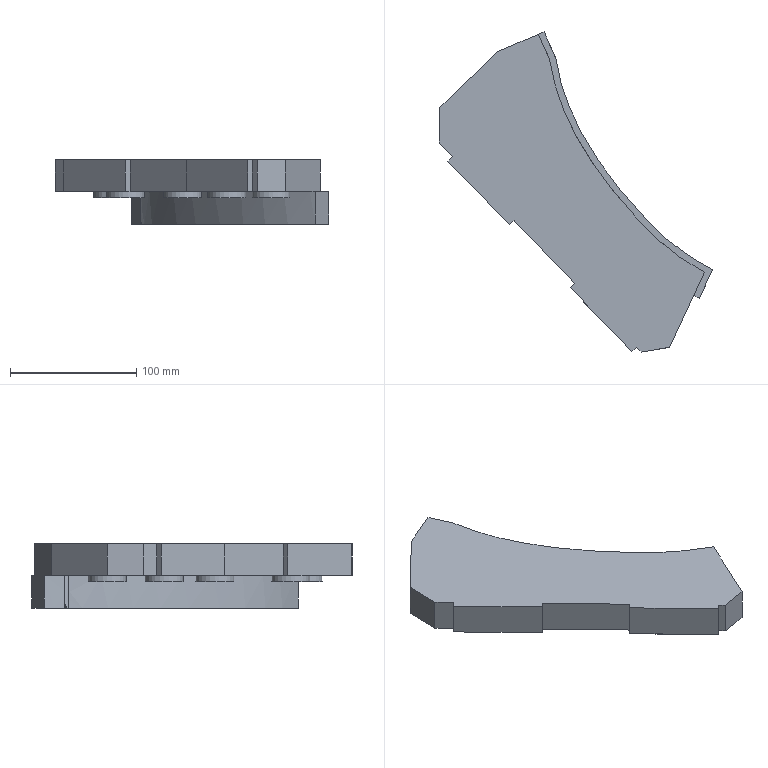Part | NX | features solid 2 | 1 solid | 32 faces | box 216.104 x 253.124 x 51 mm | volume 711831 mm3 | plane 24 | cylinder 5 | spline 3 | commonest cylinder face diameters 30 x5
STEP:
#1=CARTESIAN_POINT('',(-720.611,-200.558,20.));
#2=VERTEX_POINT('',#1);
#3=CARTESIAN_POINT('',(-705.611,-200.558,20.));
#4=DIRECTION('',(0.,0.,-1.));
#5=DIRECTION('',(-1.,0.,0.));
#6=AXIS2_PLACEMENT_3D('',#3,#4,#5);
#7=CIRCLE('',#6,15.);
#8=EDGE_CURVE('',#2,#2,#7,.T.);
#9=ORIENTED_EDGE('',*,*,#8,.F.);
#10=EDGE_LOOP('',(#9));
#11=FACE_BOUND('',#10,.T.);
#12=CARTESIAN_POINT('',(-640.003,-204.168,20.));
#13=VERTEX_POINT('',#12);
#14=CARTESIAN_POINT('',(-659.197,-245.33,20.));
#15=VERTEX_POINT('',#14);
#16=CARTESIAN_POINT('',(-631.647,-186.248,20.));
#17=DIRECTION('',(0.4226,0.9063,0.));
#18=VECTOR('',#17,1000.);
#19=LINE('',#16,#18);
#20=EDGE_CURVE('',#13,#15,#19,.F.);
#21=ORIENTED_EDGE('',*,*,#20,.T.);
#22=CARTESIAN_POINT('',(-681.543,-249.069,20.));
#23=VERTEX_POINT('',#22);
#24=CARTESIAN_POINT('',(-659.197,-245.33,20.));
#25=DIRECTION('',(0.9863,0.165,0.));
#26=VECTOR('',#25,1000.);
#27=LINE('',#24,#26);
#28=EDGE_CURVE('',#15,#23,#27,.F.);
#29=ORIENTED_EDGE('',*,*,#28,.T.);
#30=CARTESIAN_POINT('',(-685.314,-245.163,20.));
#31=VERTEX_POINT('',#30);
#32=CARTESIAN_POINT('',(-646.435,-285.424,20.));
#33=DIRECTION('',(0.6947,-0.7193,0.));
#34=VECTOR('',#33,1000.);
#35=LINE('',#32,#34);
#36=EDGE_CURVE('',#23,#31,#35,.F.);
#37=ORIENTED_EDGE('',*,*,#36,.T.);
#38=CARTESIAN_POINT('',(-688.911,-248.636,20.));
#39=VERTEX_POINT('',#38);
#40=CARTESIAN_POINT('',(-604.539,-167.159,20.));
#41=DIRECTION('',(0.7193,0.6947,0.));
#42=VECTOR('',#41,1000.);
#43=LINE('',#40,#42);
#44=EDGE_CURVE('',#31,#39,#43,.F.);
#45=ORIENTED_EDGE('',*,*,#44,.T.);
#46=CARTESIAN_POINT('',(-737.537,-198.283,20.));
#47=VERTEX_POINT('',#46);
#48=CARTESIAN_POINT('',(-661.125,-277.41,20.));
#49=DIRECTION('',(0.6947,-0.7193,0.));
#50=VECTOR('',#49,1000.);
#51=LINE('',#48,#50);
#52=EDGE_CURVE('',#47,#39,#51,.T.);
#53=ORIENTED_EDGE('',*,*,#52,.F.);
#54=CARTESIAN_POINT('',(-733.94,-194.809,20.));
#55=VERTEX_POINT('',#54);
#56=CARTESIAN_POINT('',(-653.165,-116.805,20.));
#57=DIRECTION('',(0.7193,0.6947,0.));
#58=VECTOR('',#57,1000.);
#59=LINE('',#56,#58);
#60=EDGE_CURVE('',#55,#47,#59,.F.);
#61=ORIENTED_EDGE('',*,*,#60,.F.);
#62=CARTESIAN_POINT('',(-782.058,-144.982,20.));
#63=VERTEX_POINT('',#62);
#64=CARTESIAN_POINT('',(-646.435,-285.424,20.));
#65=DIRECTION('',(0.6947,-0.7193,0.));
#66=VECTOR('',#65,1000.);
#67=LINE('',#64,#66);
#68=EDGE_CURVE('',#55,#63,#67,.F.);
#69=ORIENTED_EDGE('',*,*,#68,.T.);
#70=CARTESIAN_POINT('',(-785.655,-148.455,20.));
#71=VERTEX_POINT('',#70);
#72=CARTESIAN_POINT('',(-701.283,-66.978,20.));
#73=DIRECTION('',(0.7193,0.6947,0.));
#74=VECTOR('',#73,1000.);
#75=LINE('',#72,#74);
#76=EDGE_CURVE('',#63,#71,#75,.F.);
#77=ORIENTED_EDGE('',*,*,#76,.T.);
#78=CARTESIAN_POINT('',(-834.281,-98.101,20.));
#79=VERTEX_POINT('',#78);
#80=CARTESIAN_POINT('',(-837.754,-94.505,20.));
#81=DIRECTION('',(0.6947,-0.7193,0.));
#82=VECTOR('',#81,1000.);
#83=LINE('',#80,#82);
#84=EDGE_CURVE('',#79,#71,#83,.T.);
#85=ORIENTED_EDGE('',*,*,#84,.F.);
#86=CARTESIAN_POINT('',(-830.684,-94.628,20.));
#87=VERTEX_POINT('',#86);
#88=CARTESIAN_POINT('',(-749.909,-16.624,20.));
#89=DIRECTION('',(0.7193,0.6947,0.));
#90=VECTOR('',#89,1000.);
#91=LINE('',#88,#90);
#92=EDGE_CURVE('',#87,#79,#91,.F.);
#93=ORIENTED_EDGE('',*,*,#92,.F.);
#94=CARTESIAN_POINT('',(-841.104,-83.838,20.));
#95=VERTEX_POINT('',#94);
#96=CARTESIAN_POINT('',(-646.435,-285.424,20.));
#97=DIRECTION('',(0.6947,-0.7193,0.));
#98=VECTOR('',#97,1000.);
#99=LINE('',#96,#98);
#100=EDGE_CURVE('',#87,#95,#99,.F.);
#101=ORIENTED_EDGE('',*,*,#100,.T.);
#102=CARTESIAN_POINT('',(-840.611,-55.558,20.));
#103=VERTEX_POINT('',#102);
#104=CARTESIAN_POINT('',(-841.104,-83.838,20.));
#105=DIRECTION('',(0.01745,0.9998,0.));
#106=VECTOR('',#105,1000.);
#107=LINE('',#104,#106);
#108=EDGE_CURVE('',#95,#103,#107,.T.);
#109=ORIENTED_EDGE('',*,*,#108,.T.);
#110=CARTESIAN_POINT('',(-795.068,-11.578,20.));
#111=VERTEX_POINT('',#110);
#112=CARTESIAN_POINT('',(-774.222,8.553,20.));
#113=DIRECTION('',(-0.7193,-0.6947,0.));
#114=VECTOR('',#113,1000.);
#115=LINE('',#112,#114);
#116=EDGE_CURVE('',#103,#111,#115,.F.);
#117=ORIENTED_EDGE('',*,*,#116,.T.);
#118=CARTESIAN_POINT('',(-781.258,-5.716,20.));
#119=VERTEX_POINT('',#118);
#120=CARTESIAN_POINT('',(-1958.229,-505.311,20.));
#121=DIRECTION('',(-0.9205,-0.3907,0.));
#122=VECTOR('',#121,1000.);
#123=LINE('',#120,#122);
#124=EDGE_CURVE('',#111,#119,#123,.F.);
#125=ORIENTED_EDGE('',*,*,#124,.T.);
#126=CARTESIAN_POINT('',(-640.003,-204.168,20.));
#127=CARTESIAN_POINT('',(-649.16,-199.229,20.));
#128=CARTESIAN_POINT('',(-658.155,-193.671,20.));
#129=CARTESIAN_POINT('',(-674.999,-181.298,20.));
#130=CARTESIAN_POINT('',(-682.803,-174.446,20.));
#131=CARTESIAN_POINT('',(-697.433,-159.689,20.));
#132=CARTESIAN_POINT('',(-704.434,-151.972,20.));
#133=CARTESIAN_POINT('',(-718.006,-136.075,20.));
#134=CARTESIAN_POINT('',(-724.478,-127.917,20.));
#135=CARTESIAN_POINT('',(-736.62,-111.085,20.));
#136=CARTESIAN_POINT('',(-742.292,-102.411,20.));
#137=CARTESIAN_POINT('',(-752.624,-84.404,20.));
#138=CARTESIAN_POINT('',(-757.308,-75.035,20.));
#139=CARTESIAN_POINT('',(-765.276,-55.633,20.));
#140=CARTESIAN_POINT('',(-768.539,-45.674,20.));
#141=CARTESIAN_POINT('',(-771.484,-32.818,20.));
#142=CARTESIAN_POINT('',(-772.016,-30.226,20.));
#143=CARTESIAN_POINT('',(-772.603,-26.959,20.));
#144=CARTESIAN_POINT('',(-772.774,-25.976,20.));
#145=CARTESIAN_POINT('',(-772.936,-24.991,20.));
#146=CARTESIAN_POINT('',(-773.042,-24.334,20.));
#147=CARTESIAN_POINT('',(-773.052,-23.989,20.));
#148=CARTESIAN_POINT('',(-773.753,-22.502,20.));
#149=CARTESIAN_POINT('',(-774.301,-21.307,20.));
#150=CARTESIAN_POINT('',(-777.083,-15.349,20.));
#151=CARTESIAN_POINT('',(-779.311,-10.583,20.));
#152=CARTESIAN_POINT('',(-781.258,-5.716,20.));
#153=B_SPLINE_CURVE_WITH_KNOTS('',3,(#126,#127,#128,#129,#130,#131,#132,#133,#134,#135,#136,#137,#138,#139,#140,#141,#142,#143,#144,#145,#146,#147,#148,#149,#150,#151,#152),.UNSPECIFIED.,.F.,.F.,(4,2,2,2,2,2,2,2,2,1,2,2,2,4),(0.,0.125,0.25,0.375,0.5,0.625,0.75,0.875,0.9062,0.9141,0.918,0.9219,0.9375,1.),.UNSPECIFIED.);
#154=EDGE_CURVE('',#13,#119,#153,.T.);
#155=ORIENTED_EDGE('',*,*,#154,.F.);
#156=EDGE_LOOP('',(#21,#29,#37,#45,#53,#61,#69,#77,#85,#93,#101,#109,#117,#125,#155));
#157=FACE_BOUND('',#156,.T.);
#158=CARTESIAN_POINT('',(-770.611,-100.558,20.));
#159=VERTEX_POINT('',#158);
#160=CARTESIAN_POINT('',(-785.611,-100.558,20.));
#161=DIRECTION('',(0.,0.,1.));
#162=DIRECTION('',(1.,0.,0.));
#163=AXIS2_PLACEMENT_3D('',#160,#161,#162);
#164=CIRCLE('',#163,15.);
#165=EDGE_CURVE('',#159,#159,#164,.T.);
#166=ORIENTED_EDGE('',*,*,#165,.T.);
#167=EDGE_LOOP('',(#166));
#168=FACE_BOUND('',#167,.T.);
#169=CARTESIAN_POINT('',(-780.611,-55.558,20.));
#170=VERTEX_POINT('',#169);
#171=CARTESIAN_POINT('',(-795.611,-55.558,20.));
#172=DIRECTION('',(0.,0.,1.));
#173=DIRECTION('',(1.,0.,0.));
#174=AXIS2_PLACEMENT_3D('',#171,#172,#173);
#175=CIRCLE('',#174,15.);
#176=EDGE_CURVE('',#170,#170,#175,.T.);
#177=ORIENTED_EDGE('',*,*,#176,.T.);
#178=EDGE_LOOP('',(#177));
#179=FACE_BOUND('',#178,.T.);
#180=CARTESIAN_POINT('',(-755.611,-140.558,20.));
#181=VERTEX_POINT('',#180);
#182=CARTESIAN_POINT('',(-740.611,-140.558,20.));
#183=DIRECTION('',(0.,0.,-1.));
#184=DIRECTION('',(-1.,0.,0.));
#185=AXIS2_PLACEMENT_3D('',#182,#183,#184);
#186=CIRCLE('',#185,15.);
#187=EDGE_CURVE('',#181,#181,#186,.T.);
#188=ORIENTED_EDGE('',*,*,#187,.F.);
#189=EDGE_LOOP('',(#188));
#190=FACE_BOUND('',#189,.T.);
#191=CARTESIAN_POINT('',(-685.611,-210.558,20.));
#192=VERTEX_POINT('',#191);
#193=CARTESIAN_POINT('',(-670.611,-210.558,20.));
#194=DIRECTION('',(0.,0.,-1.));
#195=DIRECTION('',(-1.,0.,0.));
#196=AXIS2_PLACEMENT_3D('',#193,#194,#195);
#197=CIRCLE('',#196,15.);
#198=EDGE_CURVE('',#192,#192,#197,.T.);
#199=ORIENTED_EDGE('',*,*,#198,.F.);
#200=EDGE_LOOP('',(#199));
#201=FACE_BOUND('',#200,.T.);
#202=CARTESIAN_POINT('',(-565.659,-207.42,20.));
#203=DIRECTION('',(0.,0.,-1.));
#204=DIRECTION('',(-1.,0.,0.));
#205=AXIS2_PLACEMENT_3D('',#202,#203,#204);
#206=PLANE('',#205);
#207=ADVANCED_FACE('',(#11,#157,#168,#179,#190,#201),#206,.T.);
#208=CARTESIAN_POINT('',(-631.535,-186.008,20.));
#209=VERTEX_POINT('',#208);
#210=CARTESIAN_POINT('',(-631.535,-186.008,45.));
#211=VERTEX_POINT('',#210);
#212=CARTESIAN_POINT('',(-631.535,-186.008,32.5));
#213=DIRECTION('',(0.,0.,-1.));
#214=VECTOR('',#213,1000.);
#215=LINE('',#212,#214);
#216=EDGE_CURVE('',#209,#211,#215,.F.);
#217=ORIENTED_EDGE('',*,*,#216,.F.);
#218=CARTESIAN_POINT('',(-762.843,2.1,20.));
#219=VERTEX_POINT('',#218);
#220=CARTESIAN_POINT('',(-631.535,-186.008,20.));
#221=CARTESIAN_POINT('',(-635.789,-183.687,20.));
#222=CARTESIAN_POINT('',(-644.159,-178.788,20.));
#223=CARTESIAN_POINT('',(-656.221,-170.521,20.));
#224=CARTESIAN_POINT('',(-667.69,-161.153,20.));
#225=CARTESIAN_POINT('',(-678.201,-150.812,20.));
#226=CARTESIAN_POINT('',(-688.244,-139.998,20.));
#227=CARTESIAN_POINT('',(-701.112,-125.267,20.));
#228=CARTESIAN_POINT('',(-713.112,-109.922,20.));
#229=CARTESIAN_POINT('',(-723.992,-93.811,20.));
#230=CARTESIAN_POINT('',(-731.511,-81.281,20.));
#231=CARTESIAN_POINT('',(-738.298,-68.261,20.));
#232=CARTESIAN_POINT('',(-743.263,-56.884,20.));
#233=CARTESIAN_POINT('',(-746.689,-47.546,20.));
#234=CARTESIAN_POINT('',(-748.961,-40.442,20.));
#235=CARTESIAN_POINT('',(-750.591,-34.427,20.));
#236=CARTESIAN_POINT('',(-751.722,-29.553,20.));
#237=CARTESIAN_POINT('',(-752.488,-25.868,20.));
#238=CARTESIAN_POINT('',(-753.027,-22.762,20.));
#239=CARTESIAN_POINT('',(-753.46,-20.278,20.));
#240=CARTESIAN_POINT('',(-753.634,-18.362,20.));
#241=CARTESIAN_POINT('',(-754.376,-16.647,20.));
#242=CARTESIAN_POINT('',(-755.479,-14.402,20.));
#243=CARTESIAN_POINT('',(-756.769,-11.564,20.));
#244=CARTESIAN_POINT('',(-758.364,-8.175,20.));
#245=CARTESIAN_POINT('',(-760.444,-3.64,20.));
#246=CARTESIAN_POINT('',(-761.927,-0.2114,20.));
#247=CARTESIAN_POINT('',(-762.843,2.1,20.));
#248=B_SPLINE_CURVE_WITH_KNOTS('',3,(#220,#221,#222,#223,#224,#225,#226,#227,#228,#229,#230,#231,#232,#233,#234,#235,#236,#237,#238,#239,#240,#241,#242,#243,#244,#245,#246,#247),.UNSPECIFIED.,.F.,.F.,(4,1,1,1,1,1,1,1,1,1,1,1,1,1,1,1,1,1,1,1,1,1,1,1,1,4),(0.7404,0.7551,0.7697,0.7844,0.7991,0.8137,0.8284,0.8577,0.8724,0.887,0.9017,0.9163,0.9237,0.931,0.9383,0.942,0.9456,0.9493,0.9511,0.953,0.9548,0.9566,0.9603,0.964,0.9676,0.975),.UNSPECIFIED.);
#249=EDGE_CURVE('',#209,#219,#248,.T.);
#250=ORIENTED_EDGE('',*,*,#249,.T.);
#251=CARTESIAN_POINT('',(-762.843,2.1,45.));
#252=VERTEX_POINT('',#251);
#253=CARTESIAN_POINT('',(-762.843,2.1,42.5));
#254=DIRECTION('',(0.,0.,-1.));
#255=VECTOR('',#254,1000.);
#256=LINE('',#253,#255);
#257=EDGE_CURVE('',#219,#252,#256,.F.);
#258=ORIENTED_EDGE('',*,*,#257,.T.);
#259=CARTESIAN_POINT('',(-631.535,-186.008,45.));
#260=CARTESIAN_POINT('',(-635.79,-183.686,45.));
#261=CARTESIAN_POINT('',(-644.175,-178.778,45.));
#262=CARTESIAN_POINT('',(-656.267,-170.491,45.));
#263=CARTESIAN_POINT('',(-667.861,-161.004,45.));
#264=CARTESIAN_POINT('',(-678.395,-150.608,45.));
#265=CARTESIAN_POINT('',(-688.433,-139.79,45.));
#266=CARTESIAN_POINT('',(-701.359,-124.97,45.));
#267=CARTESIAN_POINT('',(-713.457,-109.469,45.));
#268=CARTESIAN_POINT('',(-724.514,-93.,45.));
#269=CARTESIAN_POINT('',(-732.09,-80.249,45.));
#270=CARTESIAN_POINT('',(-738.81,-67.179,45.));
#271=CARTESIAN_POINT('',(-743.63,-55.962,45.));
#272=CARTESIAN_POINT('',(-746.951,-46.773,45.));
#273=CARTESIAN_POINT('',(-749.158,-39.765,45.));
#274=CARTESIAN_POINT('',(-750.742,-33.822,45.));
#275=CARTESIAN_POINT('',(-751.843,-28.999,45.));
#276=CARTESIAN_POINT('',(-752.584,-25.348,45.));
#277=CARTESIAN_POINT('',(-753.119,-22.271,45.));
#278=CARTESIAN_POINT('',(-753.516,-19.798,45.));
#279=CARTESIAN_POINT('',(-753.755,-17.918,45.));
#280=CARTESIAN_POINT('',(-754.577,-16.276,45.));
#281=CARTESIAN_POINT('',(-755.62,-14.066,45.));
#282=CARTESIAN_POINT('',(-756.901,-11.293,45.));
#283=CARTESIAN_POINT('',(-758.457,-7.973,45.));
#284=CARTESIAN_POINT('',(-760.493,-3.531,45.));
#285=CARTESIAN_POINT('',(-761.944,-0.169,45.));
#286=CARTESIAN_POINT('',(-762.843,2.1,45.));
#287=B_SPLINE_CURVE_WITH_KNOTS('',3,(#259,#260,#261,#262,#263,#264,#265,#266,#267,#268,#269,#270,#271,#272,#273,#274,#275,#276,#277,#278,#279,#280,#281,#282,#283,#284,#285,#286),.UNSPECIFIED.,.F.,.F.,(4,1,1,1,1,1,1,1,1,1,1,1,1,1,1,1,1,1,1,1,1,1,1,1,1,4),(0.06935,0.08388,0.09841,0.1129,0.1275,0.142,0.1565,0.1856,0.2001,0.2147,0.2292,0.2437,0.251,0.2583,0.2655,0.2692,0.2728,0.2764,0.2782,0.2801,0.2819,0.2837,0.2873,0.291,0.2946,0.3019),.UNSPECIFIED.);
#288=EDGE_CURVE('',#211,#252,#287,.T.);
#289=ORIENTED_EDGE('',*,*,#288,.F.);
#290=EDGE_LOOP('',(#217,#250,#258,#289));
#291=FACE_BOUND('',#290,.T.);
#292=CARTESIAN_POINT('',(-631.535,-186.008,45.));
#293=CARTESIAN_POINT('',(-631.535,-186.008,20.));
#294=CARTESIAN_POINT('',(-635.877,-183.639,45.));
#295=CARTESIAN_POINT('',(-635.877,-183.639,20.));
#296=CARTESIAN_POINT('',(-644.43,-178.626,45.));
#297=CARTESIAN_POINT('',(-644.43,-178.626,20.));
#298=CARTESIAN_POINT('',(-656.738,-170.143,45.));
#299=CARTESIAN_POINT('',(-656.738,-170.143,20.));
#300=CARTESIAN_POINT('',(-668.325,-160.586,45.));
#301=CARTESIAN_POINT('',(-668.325,-160.586,20.));
#302=CARTESIAN_POINT('',(-678.899,-150.079,45.));
#303=CARTESIAN_POINT('',(-678.899,-150.079,20.));
#304=CARTESIAN_POINT('',(-688.858,-139.317,45.));
#305=CARTESIAN_POINT('',(-688.858,-139.317,20.));
#306=CARTESIAN_POINT('',(-701.731,-124.516,45.));
#307=CARTESIAN_POINT('',(-701.731,-124.516,20.));
#308=CARTESIAN_POINT('',(-713.804,-108.992,45.));
#309=CARTESIAN_POINT('',(-713.804,-108.992,20.));
#310=CARTESIAN_POINT('',(-724.771,-92.591,45.));
#311=CARTESIAN_POINT('',(-724.771,-92.591,20.));
#312=CARTESIAN_POINT('',(-732.323,-79.832,45.));
#313=CARTESIAN_POINT('',(-732.323,-79.832,20.));
#314=CARTESIAN_POINT('',(-739.096,-66.587,45.));
#315=CARTESIAN_POINT('',(-739.096,-66.587,20.));
#316=CARTESIAN_POINT('',(-743.961,-55.141,45.));
#317=CARTESIAN_POINT('',(-743.961,-55.141,20.));
#318=CARTESIAN_POINT('',(-747.295,-45.752,45.));
#319=CARTESIAN_POINT('',(-747.295,-45.752,20.));
#320=CARTESIAN_POINT('',(-749.129,-39.787,45.));
#321=CARTESIAN_POINT('',(-749.129,-39.787,20.));
#322=CARTESIAN_POINT('',(-750.434,-34.959,45.));
#323=CARTESIAN_POINT('',(-750.434,-34.959,20.));
#324=CARTESIAN_POINT('',(-751.326,-31.312,45.));
#325=CARTESIAN_POINT('',(-751.326,-31.312,20.));
#326=CARTESIAN_POINT('',(-751.996,-28.253,45.));
#327=CARTESIAN_POINT('',(-751.996,-28.253,20.));
#328=CARTESIAN_POINT('',(-752.486,-25.792,45.));
#329=CARTESIAN_POINT('',(-752.486,-25.792,20.));
#330=CARTESIAN_POINT('',(-752.828,-23.947,45.));
#331=CARTESIAN_POINT('',(-752.828,-23.947,20.));
#332=CARTESIAN_POINT('',(-753.149,-22.073,45.));
#333=CARTESIAN_POINT('',(-753.149,-22.073,20.));
#334=CARTESIAN_POINT('',(-753.389,-20.598,45.));
#335=CARTESIAN_POINT('',(-753.389,-20.598,20.));
#336=CARTESIAN_POINT('',(-753.591,-19.213,45.));
#337=CARTESIAN_POINT('',(-753.591,-19.213,20.));
#338=CARTESIAN_POINT('',(-753.684,-18.555,45.));
#339=CARTESIAN_POINT('',(-753.684,-18.555,20.));
#340=CARTESIAN_POINT('',(-753.776,-18.194,45.));
#341=CARTESIAN_POINT('',(-753.776,-18.194,20.));
#342=CARTESIAN_POINT('',(-753.995,-17.507,45.));
#343=CARTESIAN_POINT('',(-753.995,-17.507,20.));
#344=CARTESIAN_POINT('',(-754.438,-16.537,45.));
#345=CARTESIAN_POINT('',(-754.438,-16.537,20.));
#346=CARTESIAN_POINT('',(-755.321,-14.712,45.));
#347=CARTESIAN_POINT('',(-755.321,-14.712,20.));
#348=CARTESIAN_POINT('',(-756.062,-13.095,45.));
#349=CARTESIAN_POINT('',(-756.062,-13.095,20.));
#350=CARTESIAN_POINT('',(-757.086,-10.905,45.));
#351=CARTESIAN_POINT('',(-757.086,-10.905,20.));
#352=CARTESIAN_POINT('',(-758.371,-8.154,45.));
#353=CARTESIAN_POINT('',(-758.371,-8.154,20.));
#354=CARTESIAN_POINT('',(-760.425,-3.686,45.));
#355=CARTESIAN_POINT('',(-760.425,-3.686,20.));
#356=CARTESIAN_POINT('',(-761.913,-0.2481,45.));
#357=CARTESIAN_POINT('',(-761.913,-0.2481,20.));
#358=CARTESIAN_POINT('',(-762.843,2.1,45.));
#359=CARTESIAN_POINT('',(-762.843,2.1,20.));
#360=B_SPLINE_SURFACE_WITH_KNOTS('',3,1,((#292,#293),(#294,#295),(#296,#297),(#298,#299),(#300,#301),(#302,#303),(#304,#305),(#306,#307),(#308,#309),(#310,#311),(#312,#313),(#314,#315),(#316,#317),(#318,#319),(#320,#321),(#322,#323),(#324,#325),(#326,#327),(#328,#329),(#330,#331),(#332,#333),(#334,#335),(#336,#337),(#338,#339),(#340,#341),(#342,#343),(#344,#345),(#346,#347),(#348,#349),(#350,#351),(#352,#353),(#354,#355),(#356,#357),(#358,#359)),.SURF_OF_LINEAR_EXTRUSION.,.F.,.F.,.F.,(4,1,1,1,1,1,1,1,1,1,1,1,1,1,1,1,1,1,1,1,1,1,1,1,1,1,1,1,1,1,1,4),(2,2),(0.2278,0.276,0.3243,0.3725,0.4208,0.469,0.5172,0.6137,0.6619,0.7102,0.7584,0.8066,0.8308,0.8549,0.8669,0.879,0.8911,0.8971,0.9031,0.9092,0.9152,0.9182,0.9212,0.9242,0.9272,0.9333,0.9393,0.9453,0.9514,0.9634,0.9755,0.9996),(0.,1.),.UNSPECIFIED.);
#361=ADVANCED_FACE('',(#291),#360,.F.);
#362=CARTESIAN_POINT('',(-681.543,-249.069,45.));
#363=VERTEX_POINT('',#362);
#364=CARTESIAN_POINT('',(-685.314,-245.163,45.));
#365=VERTEX_POINT('',#364);
#366=CARTESIAN_POINT('',(-588.334,-345.59,45.));
#367=DIRECTION('',(-0.6947,0.7193,0.));
#368=VECTOR('',#367,1000.);
#369=LINE('',#366,#368);
#370=EDGE_CURVE('',#363,#365,#369,.T.);
#371=ORIENTED_EDGE('',*,*,#370,.F.);
#372=CARTESIAN_POINT('',(-659.197,-245.33,45.));
#373=VERTEX_POINT('',#372);
#374=CARTESIAN_POINT('',(-979.512,-298.932,45.));
#375=DIRECTION('',(0.9863,0.165,0.));
#376=VECTOR('',#375,1000.);
#377=LINE('',#374,#376);
#378=EDGE_CURVE('',#363,#373,#377,.T.);
#379=ORIENTED_EDGE('',*,*,#378,.T.);
#380=CARTESIAN_POINT('',(-631.647,-186.248,45.));
#381=DIRECTION('',(0.4226,0.9063,0.));
#382=VECTOR('',#381,1000.);
#383=LINE('',#380,#382);
#384=EDGE_CURVE('',#211,#373,#383,.F.);
#385=ORIENTED_EDGE('',*,*,#384,.F.);
#386=ORIENTED_EDGE('',*,*,#288,.T.);
#387=CARTESIAN_POINT('',(-795.068,-11.578,45.));
#388=VERTEX_POINT('',#387);
#389=CARTESIAN_POINT('',(-1958.229,-505.311,45.));
#390=DIRECTION('',(0.9205,0.3907,0.));
#391=VECTOR('',#390,1000.);
#392=LINE('',#389,#391);
#393=EDGE_CURVE('',#388,#252,#392,.T.);
#394=ORIENTED_EDGE('',*,*,#393,.F.);
#395=CARTESIAN_POINT('',(-840.611,-55.558,45.));
#396=VERTEX_POINT('',#395);
#397=CARTESIAN_POINT('',(-1185.034,-388.164,45.));
#398=DIRECTION('',(0.7193,0.6947,0.));
#399=VECTOR('',#398,1000.);
#400=LINE('',#397,#399);
#401=EDGE_CURVE('',#396,#388,#400,.T.);
#402=ORIENTED_EDGE('',*,*,#401,.F.);
#403=CARTESIAN_POINT('',(-841.104,-83.838,45.));
#404=VERTEX_POINT('',#403);
#405=CARTESIAN_POINT('',(-851.257,-665.474,45.));
#406=DIRECTION('',(0.01745,0.9998,0.));
#407=VECTOR('',#406,1000.);
#408=LINE('',#405,#407);
#409=EDGE_CURVE('',#396,#404,#408,.F.);
#410=ORIENTED_EDGE('',*,*,#409,.T.);
#411=CARTESIAN_POINT('',(-830.684,-94.628,45.));
#412=VERTEX_POINT('',#411);
#413=CARTESIAN_POINT('',(-588.334,-345.59,45.));
#414=DIRECTION('',(-0.6947,0.7193,0.));
#415=VECTOR('',#414,1000.);
#416=LINE('',#413,#415);
#417=EDGE_CURVE('',#412,#404,#416,.T.);
#418=ORIENTED_EDGE('',*,*,#417,.F.);
#419=CARTESIAN_POINT('',(-834.281,-98.101,45.));
#420=VERTEX_POINT('',#419);
#421=CARTESIAN_POINT('',(-1160.721,-413.341,45.));
#422=DIRECTION('',(-0.7193,-0.6947,0.));
#423=VECTOR('',#422,1000.);
#424=LINE('',#421,#423);
#425=EDGE_CURVE('',#412,#420,#424,.T.);
#426=ORIENTED_EDGE('',*,*,#425,.T.);
#427=CARTESIAN_POINT('',(-785.655,-148.455,45.));
#428=VERTEX_POINT('',#427);
#429=CARTESIAN_POINT('',(-837.754,-94.505,45.));
#430=DIRECTION('',(0.6947,-0.7193,0.));
#431=VECTOR('',#430,1000.);
#432=LINE('',#429,#431);
#433=EDGE_CURVE('',#420,#428,#432,.T.);
#434=ORIENTED_EDGE('',*,*,#433,.T.);
#435=CARTESIAN_POINT('',(-782.058,-144.982,45.));
#436=VERTEX_POINT('',#435);
#437=CARTESIAN_POINT('',(-1112.095,-463.694,45.));
#438=DIRECTION('',(-0.7193,-0.6947,0.));
#439=VECTOR('',#438,1000.);
#440=LINE('',#437,#439);
#441=EDGE_CURVE('',#436,#428,#440,.T.);
#442=ORIENTED_EDGE('',*,*,#441,.F.);
#443=CARTESIAN_POINT('',(-733.94,-194.809,45.));
#444=VERTEX_POINT('',#443);
#445=CARTESIAN_POINT('',(-588.334,-345.59,45.));
#446=DIRECTION('',(-0.6947,0.7193,0.));
#447=VECTOR('',#446,1000.);
#448=LINE('',#445,#447);
#449=EDGE_CURVE('',#444,#436,#448,.T.);
#450=ORIENTED_EDGE('',*,*,#449,.F.);
#451=CARTESIAN_POINT('',(-737.537,-198.283,45.));
#452=VERTEX_POINT('',#451);
#453=CARTESIAN_POINT('',(-1063.977,-513.522,45.));
#454=DIRECTION('',(-0.7193,-0.6947,0.));
#455=VECTOR('',#454,1000.);
#456=LINE('',#453,#455);
#457=EDGE_CURVE('',#444,#452,#456,.T.);
#458=ORIENTED_EDGE('',*,*,#457,.T.);
#459=CARTESIAN_POINT('',(-688.911,-248.636,45.));
#460=VERTEX_POINT('',#459);
#461=CARTESIAN_POINT('',(-661.125,-277.41,45.));
#462=DIRECTION('',(0.6947,-0.7193,0.));
#463=VECTOR('',#462,1000.);
#464=LINE('',#461,#463);
#465=EDGE_CURVE('',#452,#460,#464,.T.);
#466=ORIENTED_EDGE('',*,*,#465,.T.);
#467=CARTESIAN_POINT('',(-1015.351,-563.876,45.));
#468=DIRECTION('',(-0.7193,-0.6947,0.));
#469=VECTOR('',#468,1000.);
#470=LINE('',#467,#469);
#471=EDGE_CURVE('',#365,#460,#470,.T.);
#472=ORIENTED_EDGE('',*,*,#471,.F.);
#473=EDGE_LOOP('',(#371,#379,#385,#386,#394,#402,#410,#418,#426,#434,#442,#450,#458,#466,#472));
#474=FACE_BOUND('',#473,.T.);
#475=CARTESIAN_POINT('',(-918.37,-664.302,45.));
#476=DIRECTION('',(0.,0.,1.));
#477=DIRECTION('',(1.,0.,0.));
#478=AXIS2_PLACEMENT_3D('',#475,#476,#477);
#479=PLANE('',#478);
#480=ADVANCED_FACE('',(#474),#479,.T.);
#481=ORIENTED_EDGE('',*,*,#36,.F.);
#482=CARTESIAN_POINT('',(-681.543,-249.069,45.));
#483=DIRECTION('',(0.,0.,1.));
#484=VECTOR('',#483,1000.);
#485=LINE('',#482,#484);
#486=EDGE_CURVE('',#23,#363,#485,.T.);
#487=ORIENTED_EDGE('',*,*,#486,.T.);
#488=ORIENTED_EDGE('',*,*,#370,.T.);
#489=CARTESIAN_POINT('',(-685.314,-245.163,45.));
#490=DIRECTION('',(0.,0.,-1.));
#491=VECTOR('',#490,1000.);
#492=LINE('',#489,#491);
#493=EDGE_CURVE('',#365,#31,#492,.T.);
#494=ORIENTED_EDGE('',*,*,#493,.T.);
#495=EDGE_LOOP('',(#481,#487,#488,#494));
#496=FACE_BOUND('',#495,.T.);
#497=CARTESIAN_POINT('',(-856.234,-68.171,45.));
#498=DIRECTION('',(0.7193,0.6947,0.));
#499=DIRECTION('',(0.6947,-0.7193,0.));
#500=AXIS2_PLACEMENT_3D('',#497,#498,#499);
#501=PLANE('',#500);
#502=ADVANCED_FACE('',(#496),#501,.F.);
#503=CARTESIAN_POINT('',(-780.611,-55.558,15.));
#504=VERTEX_POINT('',#503);
#505=CARTESIAN_POINT('',(-795.611,-55.558,15.));
#506=DIRECTION('',(0.,0.,1.));
#507=DIRECTION('',(1.,0.,0.));
#508=AXIS2_PLACEMENT_3D('',#505,#506,#507);
#509=CIRCLE('',#508,15.);
#510=EDGE_CURVE('',#504,#504,#509,.T.);
#511=ORIENTED_EDGE('',*,*,#510,.F.);
#512=EDGE_LOOP('',(#511));
#513=FACE_BOUND('',#512,.T.);
#514=CARTESIAN_POINT('',(-795.611,-55.558,15.));
#515=DIRECTION('',(0.,0.,1.));
#516=DIRECTION('',(1.,0.,0.));
#517=AXIS2_PLACEMENT_3D('',#514,#515,#516);
#518=PLANE('',#517);
#519=ADVANCED_FACE('',(#513),#518,.F.);
#520=CARTESIAN_POINT('',(-770.611,-100.558,15.));
#521=VERTEX_POINT('',#520);
#522=CARTESIAN_POINT('',(-785.611,-100.558,15.));
#523=DIRECTION('',(0.,0.,1.));
#524=DIRECTION('',(1.,0.,0.));
#525=AXIS2_PLACEMENT_3D('',#522,#523,#524);
#526=CIRCLE('',#525,15.);
#527=EDGE_CURVE('',#521,#521,#526,.T.);
#528=ORIENTED_EDGE('',*,*,#527,.F.);
#529=EDGE_LOOP('',(#528));
#530=FACE_BOUND('',#529,.T.);
#531=CARTESIAN_POINT('',(-785.611,-100.558,15.));
#532=DIRECTION('',(0.,0.,1.));
#533=DIRECTION('',(1.,0.,0.));
#534=AXIS2_PLACEMENT_3D('',#531,#532,#533);
#535=PLANE('',#534);
#536=ADVANCED_FACE('',(#530),#535,.F.);
#537=ORIENTED_EDGE('',*,*,#116,.F.);
#538=CARTESIAN_POINT('',(-840.611,-55.558,45.));
#539=DIRECTION('',(0.,0.,1.));
#540=VECTOR('',#539,1000.);
#541=LINE('',#538,#540);
#542=EDGE_CURVE('',#103,#396,#541,.T.);
#543=ORIENTED_EDGE('',*,*,#542,.T.);
#544=ORIENTED_EDGE('',*,*,#401,.T.);
#545=CARTESIAN_POINT('',(-795.068,-11.578,45.));
#546=DIRECTION('',(0.,0.,1.));
#547=VECTOR('',#546,1000.);
#548=LINE('',#545,#547);
#549=EDGE_CURVE('',#111,#388,#548,.T.);
#550=ORIENTED_EDGE('',*,*,#549,.F.);
#551=EDGE_LOOP('',(#537,#543,#544,#550));
#552=FACE_BOUND('',#551,.T.);
#553=CARTESIAN_POINT('',(-889.227,-102.506,45.));
#554=DIRECTION('',(0.6947,-0.7193,0.));
#555=DIRECTION('',(0.7193,0.6947,0.));
#556=AXIS2_PLACEMENT_3D('',#553,#554,#555);
#557=PLANE('',#556);
#558=ADVANCED_FACE('',(#552),#557,.F.);
#559=ORIENTED_EDGE('',*,*,#409,.F.);
#560=ORIENTED_EDGE('',*,*,#542,.F.);
#561=ORIENTED_EDGE('',*,*,#108,.F.);
#562=CARTESIAN_POINT('',(-841.104,-83.838,45.));
#563=DIRECTION('',(0.,0.,-1.));
#564=VECTOR('',#563,1000.);
#565=LINE('',#562,#564);
#566=EDGE_CURVE('',#404,#95,#565,.T.);
#567=ORIENTED_EDGE('',*,*,#566,.F.);
#568=EDGE_LOOP('',(#559,#560,#561,#567));
#569=FACE_BOUND('',#568,.T.);
#570=CARTESIAN_POINT('',(-841.104,-83.838,45.));
#571=DIRECTION('',(0.9998,-0.01745,0.));
#572=DIRECTION('',(0.01745,0.9998,0.));
#573=AXIS2_PLACEMENT_3D('',#570,#571,#572);
#574=PLANE('',#573);
#575=ADVANCED_FACE('',(#569),#574,.F.);
#576=ORIENTED_EDGE('',*,*,#100,.F.);
#577=CARTESIAN_POINT('',(-830.684,-94.628,45.));
#578=DIRECTION('',(0.,0.,-1.));
#579=VECTOR('',#578,1000.);
#580=LINE('',#577,#579);
#581=EDGE_CURVE('',#412,#87,#580,.T.);
#582=ORIENTED_EDGE('',*,*,#581,.F.);
#583=ORIENTED_EDGE('',*,*,#417,.T.);
#584=ORIENTED_EDGE('',*,*,#566,.T.);
#585=EDGE_LOOP('',(#576,#582,#583,#584));
#586=FACE_BOUND('',#585,.T.);
#587=CARTESIAN_POINT('',(-856.234,-68.171,45.));
#588=DIRECTION('',(0.7193,0.6947,0.));
#589=DIRECTION('',(0.6947,-0.7193,0.));
#590=AXIS2_PLACEMENT_3D('',#587,#588,#589);
#591=PLANE('',#590);
#592=ADVANCED_FACE('',(#586),#591,.F.);
#593=CARTESIAN_POINT('',(-834.281,-98.101,45.));
#594=DIRECTION('',(0.,0.,-1.));
#595=VECTOR('',#594,1000.);
#596=LINE('',#593,#595);
#597=EDGE_CURVE('',#420,#79,#596,.T.);
#598=ORIENTED_EDGE('',*,*,#597,.F.);
#599=ORIENTED_EDGE('',*,*,#425,.F.);
#600=ORIENTED_EDGE('',*,*,#581,.T.);
#601=ORIENTED_EDGE('',*,*,#92,.T.);
#602=EDGE_LOOP('',(#598,#599,#600,#601));
#603=FACE_BOUND('',#602,.T.);
#604=CARTESIAN_POINT('',(-830.684,-94.628,45.));
#605=DIRECTION('',(-0.6947,0.7193,0.));
#606=DIRECTION('',(-0.7193,-0.6947,0.));
#607=AXIS2_PLACEMENT_3D('',#604,#605,#606);
#608=PLANE('',#607);
#609=ADVANCED_FACE('',(#603),#608,.T.);
#610=CARTESIAN_POINT('',(-785.655,-148.455,45.));
#611=DIRECTION('',(0.,0.,-1.));
#612=VECTOR('',#611,1000.);
#613=LINE('',#610,#612);
#614=EDGE_CURVE('',#428,#71,#613,.T.);
#615=ORIENTED_EDGE('',*,*,#614,.F.);
#616=ORIENTED_EDGE('',*,*,#433,.F.);
#617=ORIENTED_EDGE('',*,*,#597,.T.);
#618=ORIENTED_EDGE('',*,*,#84,.T.);
#619=EDGE_LOOP('',(#615,#616,#617,#618));
#620=FACE_BOUND('',#619,.T.);
#621=CARTESIAN_POINT('',(-837.754,-94.505,45.));
#622=DIRECTION('',(-0.7193,-0.6947,0.));
#623=DIRECTION('',(0.,0.,-1.));
#624=AXIS2_PLACEMENT_3D('',#621,#622,#623);
#625=PLANE('',#624);
#626=ADVANCED_FACE('',(#620),#625,.T.);
#627=ORIENTED_EDGE('',*,*,#614,.T.);
#628=ORIENTED_EDGE('',*,*,#76,.F.);
#629=CARTESIAN_POINT('',(-782.058,-144.982,45.));
#630=DIRECTION('',(0.,0.,-1.));
#631=VECTOR('',#630,1000.);
#632=LINE('',#629,#631);
#633=EDGE_CURVE('',#436,#63,#632,.T.);
#634=ORIENTED_EDGE('',*,*,#633,.F.);
#635=ORIENTED_EDGE('',*,*,#441,.T.);
#636=EDGE_LOOP('',(#627,#628,#634,#635));
#637=FACE_BOUND('',#636,.T.);
#638=CARTESIAN_POINT('',(-782.058,-144.982,45.));
#639=DIRECTION('',(-0.6947,0.7193,0.));
#640=DIRECTION('',(-0.7193,-0.6947,0.));
#641=AXIS2_PLACEMENT_3D('',#638,#639,#640);
#642=PLANE('',#641);
#643=ADVANCED_FACE('',(#637),#642,.F.);
#644=ORIENTED_EDGE('',*,*,#633,.T.);
#645=ORIENTED_EDGE('',*,*,#68,.F.);
#646=CARTESIAN_POINT('',(-733.94,-194.809,45.));
#647=DIRECTION('',(0.,0.,-1.));
#648=VECTOR('',#647,1000.);
#649=LINE('',#646,#648);
#650=EDGE_CURVE('',#444,#55,#649,.T.);
#651=ORIENTED_EDGE('',*,*,#650,.F.);
#652=ORIENTED_EDGE('',*,*,#449,.T.);
#653=EDGE_LOOP('',(#644,#645,#651,#652));
#654=FACE_BOUND('',#653,.T.);
#655=CARTESIAN_POINT('',(-856.234,-68.171,45.));
#656=DIRECTION('',(0.7193,0.6947,0.));
#657=DIRECTION('',(0.6947,-0.7193,0.));
#658=AXIS2_PLACEMENT_3D('',#655,#656,#657);
#659=PLANE('',#658);
#660=ADVANCED_FACE('',(#654),#659,.F.);
#661=CARTESIAN_POINT('',(-737.537,-198.283,45.));
#662=DIRECTION('',(0.,0.,-1.));
#663=VECTOR('',#662,1000.);
#664=LINE('',#661,#663);
#665=EDGE_CURVE('',#452,#47,#664,.T.);
#666=ORIENTED_EDGE('',*,*,#665,.F.);
#667=ORIENTED_EDGE('',*,*,#457,.F.);
#668=ORIENTED_EDGE('',*,*,#650,.T.);
#669=ORIENTED_EDGE('',*,*,#60,.T.);
#670=EDGE_LOOP('',(#666,#667,#668,#669));
#671=FACE_BOUND('',#670,.T.);
#672=CARTESIAN_POINT('',(-733.94,-194.809,45.));
#673=DIRECTION('',(-0.6947,0.7193,0.));
#674=DIRECTION('',(-0.7193,-0.6947,0.));
#675=AXIS2_PLACEMENT_3D('',#672,#673,#674);
#676=PLANE('',#675);
#677=ADVANCED_FACE('',(#671),#676,.T.);
#678=CARTESIAN_POINT('',(-688.911,-248.636,45.));
#679=DIRECTION('',(0.,0.,-1.));
#680=VECTOR('',#679,1000.);
#681=LINE('',#678,#680);
#682=EDGE_CURVE('',#460,#39,#681,.T.);
#683=ORIENTED_EDGE('',*,*,#682,.F.);
#684=ORIENTED_EDGE('',*,*,#465,.F.);
#685=ORIENTED_EDGE('',*,*,#665,.T.);
#686=ORIENTED_EDGE('',*,*,#52,.T.);
#687=EDGE_LOOP('',(#683,#684,#685,#686));
#688=FACE_BOUND('',#687,.T.);
#689=CARTESIAN_POINT('',(-661.125,-277.41,45.));
#690=DIRECTION('',(-0.7193,-0.6947,0.));
#691=DIRECTION('',(0.,0.,-1.));
#692=AXIS2_PLACEMENT_3D('',#689,#690,#691);
#693=PLANE('',#692);
#694=ADVANCED_FACE('',(#688),#693,.T.);
#695=ORIENTED_EDGE('',*,*,#682,.T.);
#696=ORIENTED_EDGE('',*,*,#44,.F.);
#697=ORIENTED_EDGE('',*,*,#493,.F.);
#698=ORIENTED_EDGE('',*,*,#471,.T.);
#699=EDGE_LOOP('',(#695,#696,#697,#698));
#700=FACE_BOUND('',#699,.T.);
#701=CARTESIAN_POINT('',(-685.314,-245.163,45.));
#702=DIRECTION('',(-0.6947,0.7193,0.));
#703=DIRECTION('',(-0.7193,-0.6947,0.));
#704=AXIS2_PLACEMENT_3D('',#701,#702,#703);
#705=PLANE('',#704);
#706=ADVANCED_FACE('',(#700),#705,.F.);
#707=ORIENTED_EDGE('',*,*,#510,.T.);
#708=EDGE_LOOP('',(#707));
#709=FACE_BOUND('',#708,.T.);
#710=ORIENTED_EDGE('',*,*,#176,.F.);
#711=EDGE_LOOP('',(#710));
#712=FACE_BOUND('',#711,.T.);
#713=CARTESIAN_POINT('',(-795.611,-55.558,15.));
#714=DIRECTION('',(0.,0.,1.));
#715=DIRECTION('',(1.,0.,0.));
#716=AXIS2_PLACEMENT_3D('',#713,#714,#715);
#717=CYLINDRICAL_SURFACE('',#716,15.);
#718=ADVANCED_FACE('',(#709,#712),#717,.T.);
#719=ORIENTED_EDGE('',*,*,#527,.T.);
#720=EDGE_LOOP('',(#719));
#721=FACE_BOUND('',#720,.T.);
#722=ORIENTED_EDGE('',*,*,#165,.F.);
#723=EDGE_LOOP('',(#722));
#724=FACE_BOUND('',#723,.T.);
#725=CARTESIAN_POINT('',(-785.611,-100.558,15.));
#726=DIRECTION('',(0.,0.,1.));
#727=DIRECTION('',(1.,0.,0.));
#728=AXIS2_PLACEMENT_3D('',#725,#726,#727);
#729=CYLINDRICAL_SURFACE('',#728,15.);
#730=ADVANCED_FACE('',(#721,#724),#729,.T.);
#731=ORIENTED_EDGE('',*,*,#549,.T.);
#732=ORIENTED_EDGE('',*,*,#393,.T.);
#733=ORIENTED_EDGE('',*,*,#257,.F.);
#734=CARTESIAN_POINT('',(-758.239,4.055,20.));
#735=VERTEX_POINT('',#734);
#736=CARTESIAN_POINT('',(-1958.229,-505.311,20.));
#737=DIRECTION('',(0.9205,0.3907,0.));
#738=VECTOR('',#737,1000.);
#739=LINE('',#736,#738);
#740=EDGE_CURVE('',#735,#219,#739,.F.);
#741=ORIENTED_EDGE('',*,*,#740,.F.);
#742=CARTESIAN_POINT('',(-758.239,4.055,-6.));
#743=VERTEX_POINT('',#742);
#744=CARTESIAN_POINT('',(-758.239,4.055,70.));
#745=DIRECTION('',(0.,0.,-1.));
#746=VECTOR('',#745,1000.);
#747=LINE('',#744,#746);
#748=EDGE_CURVE('',#735,#743,#747,.T.);
#749=ORIENTED_EDGE('',*,*,#748,.T.);
#750=CARTESIAN_POINT('',(-781.258,-5.716,-6.));
#751=VERTEX_POINT('',#750);
#752=CARTESIAN_POINT('',(-1958.229,-505.311,-6.));
#753=DIRECTION('',(0.9205,0.3907,0.));
#754=VECTOR('',#753,1000.);
#755=LINE('',#752,#754);
#756=EDGE_CURVE('',#751,#743,#755,.T.);
#757=ORIENTED_EDGE('',*,*,#756,.F.);
#758=CARTESIAN_POINT('',(-781.258,-5.716,19.5));
#759=DIRECTION('',(0.,0.,1.));
#760=VECTOR('',#759,1000.);
#761=LINE('',#758,#760);
#762=EDGE_CURVE('',#119,#751,#761,.F.);
#763=ORIENTED_EDGE('',*,*,#762,.F.);
#764=ORIENTED_EDGE('',*,*,#124,.F.);
#765=EDGE_LOOP('',(#731,#732,#733,#741,#749,#757,#763,#764));
#766=FACE_BOUND('',#765,.T.);
#767=CARTESIAN_POINT('',(-1958.229,-505.311,70.));
#768=DIRECTION('',(-0.3907,0.9205,0.));
#769=DIRECTION('',(-0.9205,-0.3907,0.));
#770=AXIS2_PLACEMENT_3D('',#767,#768,#769);
#771=PLANE('',#770);
#772=ADVANCED_FACE('',(#766),#771,.T.);
#773=CARTESIAN_POINT('',(-635.575,-206.502,-6.));
#774=VERTEX_POINT('',#773);
#775=CARTESIAN_POINT('',(-635.575,-206.502,-6.));
#776=CARTESIAN_POINT('',(-645.074,-201.606,-6.));
#777=CARTESIAN_POINT('',(-663.823,-190.597,-6.));
#778=CARTESIAN_POINT('',(-688.155,-170.004,-6.));
#779=CARTESIAN_POINT('',(-709.387,-146.602,-6.));
#780=CARTESIAN_POINT('',(-736.036,-113.759,-6.));
#781=CARTESIAN_POINT('',(-755.461,-81.426,-6.));
#782=CARTESIAN_POINT('',(-766.657,-51.401,-6.));
#783=CARTESIAN_POINT('',(-770.316,-38.576,-6.));
#784=CARTESIAN_POINT('',(-772.026,-30.009,-6.));
#785=CARTESIAN_POINT('',(-772.796,-26.049,-6.));
#786=CARTESIAN_POINT('',(-772.943,-24.339,-6.));
#787=CARTESIAN_POINT('',(-773.352,-23.247,-6.));
#788=CARTESIAN_POINT('',(-773.087,-22.452,-6.));
#789=CARTESIAN_POINT('',(-773.982,-22.363,-6.));
#790=CARTESIAN_POINT('',(-773.,-21.784,-6.));
#791=CARTESIAN_POINT('',(-774.136,-22.086,-6.));
#792=CARTESIAN_POINT('',(-773.815,-21.844,-6.));
#793=CARTESIAN_POINT('',(-774.3,-21.724,-6.));
#794=CARTESIAN_POINT('',(-774.267,-21.096,-6.));
#795=CARTESIAN_POINT('',(-776.082,-18.375,-6.));
#796=CARTESIAN_POINT('',(-777.982,-13.042,-6.));
#797=CARTESIAN_POINT('',(-780.267,-8.193,-6.));
#798=CARTESIAN_POINT('',(-781.258,-5.716,-6.));
#799=B_SPLINE_CURVE_WITH_KNOTS('',3,(#775,#776,#777,#778,#779,#780,#781,#782,#783,#784,#785,#786,#787,#788,#789,#790,#791,#792,#793,#794,#795,#796,#797,#798),.UNSPECIFIED.,.F.,.F.,(4,1,1,1,1,1,1,1,1,1,1,1,1,1,1,1,1,1,1,1,1,4),(0.06729,0.0993,0.1313,0.1633,0.1953,0.2594,0.2754,0.2914,0.2994,0.3014,0.3034,0.3044,0.3049,0.3054,0.3055,0.3056,0.3056,0.3059,0.3064,0.3074,0.3154,0.3234),.UNSPECIFIED.);
#800=EDGE_CURVE('',#774,#751,#799,.T.);
#801=ORIENTED_EDGE('',*,*,#800,.F.);
#802=CARTESIAN_POINT('',(-635.575,-206.502,20.));
#803=VERTEX_POINT('',#802);
#804=CARTESIAN_POINT('',(-635.575,-206.502,7.));
#805=DIRECTION('',(0.,0.,1.));
#806=VECTOR('',#805,1000.);
#807=LINE('',#804,#806);
#808=EDGE_CURVE('',#774,#803,#807,.T.);
#809=ORIENTED_EDGE('',*,*,#808,.T.);
#810=CARTESIAN_POINT('',(-635.575,-206.502,20.));
#811=CARTESIAN_POINT('',(-637.057,-205.738,20.));
#812=CARTESIAN_POINT('',(-638.533,-204.96,20.));
#813=CARTESIAN_POINT('',(-640.003,-204.168,20.));
#814=B_SPLINE_CURVE_WITH_KNOTS('',3,(#810,#811,#812,#813),.UNSPECIFIED.,.F.,.F.,(4,4),(0.6105,0.6156),.UNSPECIFIED.);
#815=EDGE_CURVE('',#803,#13,#814,.T.);
#816=ORIENTED_EDGE('',*,*,#815,.T.);
#817=ORIENTED_EDGE('',*,*,#154,.T.);
#818=ORIENTED_EDGE('',*,*,#762,.T.);
#819=EDGE_LOOP('',(#801,#809,#816,#817,#818));
#820=FACE_BOUND('',#819,.T.);
#821=CARTESIAN_POINT('',(-635.575,-206.502,-6.));
#822=CARTESIAN_POINT('',(-635.575,-206.502,20.));
#823=CARTESIAN_POINT('',(-640.421,-204.004,-6.));
#824=CARTESIAN_POINT('',(-640.421,-204.004,20.));
#825=CARTESIAN_POINT('',(-650.026,-198.69,-6.));
#826=CARTESIAN_POINT('',(-650.026,-198.69,20.));
#827=CARTESIAN_POINT('',(-664.124,-189.547,-6.));
#828=CARTESIAN_POINT('',(-664.124,-189.547,20.));
#829=CARTESIAN_POINT('',(-677.678,-179.055,-6.));
#830=CARTESIAN_POINT('',(-677.678,-179.055,20.));
#831=CARTESIAN_POINT('',(-690.181,-167.239,-6.));
#832=CARTESIAN_POINT('',(-690.181,-167.239,20.));
#833=CARTESIAN_POINT('',(-700.866,-155.845,-6.));
#834=CARTESIAN_POINT('',(-700.866,-155.845,20.));
#835=CARTESIAN_POINT('',(-711.303,-144.077,-6.));
#836=CARTESIAN_POINT('',(-711.303,-144.077,20.));
#837=CARTESIAN_POINT('',(-721.358,-131.854,-6.));
#838=CARTESIAN_POINT('',(-721.358,-131.854,20.));
#839=CARTESIAN_POINT('',(-730.992,-119.104,-6.));
#840=CARTESIAN_POINT('',(-730.992,-119.104,20.));
#841=CARTESIAN_POINT('',(-740.1,-105.777,-6.));
#842=CARTESIAN_POINT('',(-740.1,-105.777,20.));
#843=CARTESIAN_POINT('',(-748.563,-91.81,-6.));
#844=CARTESIAN_POINT('',(-748.563,-91.81,20.));
#845=CARTESIAN_POINT('',(-754.954,-79.615,-6.));
#846=CARTESIAN_POINT('',(-754.954,-79.615,20.));
#847=CARTESIAN_POINT('',(-759.594,-69.486,-6.));
#848=CARTESIAN_POINT('',(-759.594,-69.486,20.));
#849=CARTESIAN_POINT('',(-762.805,-61.705,-6.));
#850=CARTESIAN_POINT('',(-762.805,-61.705,20.));
#851=CARTESIAN_POINT('',(-765.718,-53.738,-6.));
#852=CARTESIAN_POINT('',(-765.718,-53.738,20.));
#853=CARTESIAN_POINT('',(-767.873,-46.948,-6.));
#854=CARTESIAN_POINT('',(-767.873,-46.948,20.));
#855=CARTESIAN_POINT('',(-769.418,-41.419,-6.));
#856=CARTESIAN_POINT('',(-769.418,-41.419,20.));
#857=CARTESIAN_POINT('',(-770.483,-37.225,-6.));
#858=CARTESIAN_POINT('',(-770.483,-37.225,20.));
#859=CARTESIAN_POINT('',(-771.287,-33.69,-6.));
#860=CARTESIAN_POINT('',(-771.287,-33.69,20.));
#861=CARTESIAN_POINT('',(-771.877,-30.841,-6.));
#862=CARTESIAN_POINT('',(-771.877,-30.841,20.));
#863=CARTESIAN_POINT('',(-772.224,-29.049,-6.));
#864=CARTESIAN_POINT('',(-772.224,-29.049,20.));
#865=CARTESIAN_POINT('',(-772.486,-27.614,-6.));
#866=CARTESIAN_POINT('',(-772.486,-27.614,20.));
#867=CARTESIAN_POINT('',(-772.676,-26.54,-6.));
#868=CARTESIAN_POINT('',(-772.676,-26.54,20.));
#869=CARTESIAN_POINT('',(-772.858,-25.468,-6.));
#870=CARTESIAN_POINT('',(-772.858,-25.468,20.));
#871=CARTESIAN_POINT('',(-773.004,-24.575,-6.));
#872=CARTESIAN_POINT('',(-773.004,-24.575,20.));
#873=CARTESIAN_POINT('',(-773.116,-23.864,-6.));
#874=CARTESIAN_POINT('',(-773.116,-23.864,20.));
#875=CARTESIAN_POINT('',(-773.2,-23.324,-6.));
#876=CARTESIAN_POINT('',(-773.2,-23.324,20.));
#877=CARTESIAN_POINT('',(-773.287,-22.753,-6.));
#878=CARTESIAN_POINT('',(-773.287,-22.753,20.));
#879=CARTESIAN_POINT('',(-773.393,-22.011,-6.));
#880=CARTESIAN_POINT('',(-773.393,-22.011,20.));
#881=CARTESIAN_POINT('',(-773.429,-21.766,-6.));
#882=CARTESIAN_POINT('',(-773.429,-21.766,20.));
#883=CARTESIAN_POINT('',(-773.361,-22.22,-6.));
#884=CARTESIAN_POINT('',(-773.361,-22.22,20.));
#885=CARTESIAN_POINT('',(-773.184,-23.06,-6.));
#886=CARTESIAN_POINT('',(-773.184,-23.06,20.));
#887=CARTESIAN_POINT('',(-772.963,-23.882,-6.));
#888=CARTESIAN_POINT('',(-772.963,-23.882,20.));
#889=CARTESIAN_POINT('',(-772.687,-24.703,-6.));
#890=CARTESIAN_POINT('',(-772.687,-24.703,20.));
#891=CARTESIAN_POINT('',(-772.421,-25.316,-6.));
#892=CARTESIAN_POINT('',(-772.421,-25.316,20.));
#893=CARTESIAN_POINT('',(-772.489,-25.158,-6.));
#894=CARTESIAN_POINT('',(-772.489,-25.158,20.));
#895=CARTESIAN_POINT('',(-772.719,-24.685,-6.));
#896=CARTESIAN_POINT('',(-772.719,-24.685,20.));
#897=CARTESIAN_POINT('',(-773.084,-23.925,-6.));
#898=CARTESIAN_POINT('',(-773.084,-23.925,20.));
#899=CARTESIAN_POINT('',(-773.487,-23.065,-6.));
#900=CARTESIAN_POINT('',(-773.487,-23.065,20.));
#901=CARTESIAN_POINT('',(-773.898,-22.176,-6.));
#902=CARTESIAN_POINT('',(-773.898,-22.176,20.));
#903=CARTESIAN_POINT('',(-774.263,-21.39,-6.));
#904=CARTESIAN_POINT('',(-774.263,-21.39,20.));
#905=CARTESIAN_POINT('',(-774.776,-20.291,-6.));
#906=CARTESIAN_POINT('',(-774.776,-20.291,20.));
#907=CARTESIAN_POINT('',(-775.426,-18.9,-6.));
#908=CARTESIAN_POINT('',(-775.426,-18.9,20.));
#909=CARTESIAN_POINT('',(-776.23,-17.176,-6.));
#910=CARTESIAN_POINT('',(-776.23,-17.176,20.));
#911=CARTESIAN_POINT('',(-777.05,-15.405,-6.));
#912=CARTESIAN_POINT('',(-777.05,-15.405,20.));
#913=CARTESIAN_POINT('',(-778.162,-12.973,-6.));
#914=CARTESIAN_POINT('',(-778.162,-12.973,20.));
#915=CARTESIAN_POINT('',(-779.575,-9.799,-6.));
#916=CARTESIAN_POINT('',(-779.575,-9.799,20.));
#917=CARTESIAN_POINT('',(-780.702,-7.105,-6.));
#918=CARTESIAN_POINT('',(-780.702,-7.105,20.));
#919=CARTESIAN_POINT('',(-781.258,-5.716,-6.));
#920=CARTESIAN_POINT('',(-781.258,-5.716,20.));
#921=B_SPLINE_SURFACE_WITH_KNOTS('',3,1,((#821,#822),(#823,#824),(#825,#826),(#827,#828),(#829,#830),(#831,#832),(#833,#834),(#835,#836),(#837,#838),(#839,#840),(#841,#842),(#843,#844),(#845,#846),(#847,#848),(#849,#850),(#851,#852),(#853,#854),(#855,#856),(#857,#858),(#859,#860),(#861,#862),(#863,#864),(#865,#866),(#867,#868),(#869,#870),(#871,#872),(#873,#874),(#875,#876),(#877,#878),(#879,#880),(#881,#882),(#883,#884),(#885,#886),(#887,#888),(#889,#890),(#891,#892),(#893,#894),(#895,#896),(#897,#898),(#899,#900),(#901,#902),(#903,#904),(#905,#906),(#907,#908),(#909,#910),(#911,#912),(#913,#914),(#915,#916),(#917,#918),(#919,#920)),.SURF_OF_LINEAR_EXTRUSION.,.F.,.F.,.F.,(4,1,1,1,1,1,1,1,1,1,1,1,1,1,1,1,1,1,1,1,1,1,1,1,1,1,1,1,1,1,1,1,1,1,1,1,1,1,1,1,1,1,1,1,1,1,1,4),(2,2),(0.2089,0.2583,0.3076,0.3569,0.4063,0.4556,0.5049,0.5543,0.6036,0.6529,0.7023,0.7516,0.7763,0.8009,0.8256,0.8503,0.8626,0.8749,0.8873,0.8934,0.8996,0.9027,0.9058,0.9089,0.9119,0.9135,0.915,0.9166,0.9181,0.9196,0.9212,0.9227,0.9243,0.9274,0.9304,0.9335,0.9351,0.9366,0.9397,0.9428,0.9459,0.9489,0.9551,0.9613,0.9674,0.9736,0.9859,0.9983),(0.,1.),.UNSPECIFIED.);
#922=ADVANCED_FACE('',(#820),#921,.F.);
#923=CARTESIAN_POINT('',(-625.,-183.825,20.));
#924=VERTEX_POINT('',#923);
#925=CARTESIAN_POINT('',(-758.239,4.055,20.));
#926=CARTESIAN_POINT('',(-757.357,1.821,20.));
#927=CARTESIAN_POINT('',(-755.929,-1.488,20.));
#928=CARTESIAN_POINT('',(-753.925,-5.861,20.));
#929=CARTESIAN_POINT('',(-752.392,-9.129,20.));
#930=CARTESIAN_POINT('',(-751.135,-11.86,20.));
#931=CARTESIAN_POINT('',(-750.099,-14.034,20.));
#932=CARTESIAN_POINT('',(-749.323,-15.664,20.));
#933=CARTESIAN_POINT('',(-748.772,-17.383,20.));
#934=CARTESIAN_POINT('',(-748.47,-19.845,20.));
#935=CARTESIAN_POINT('',(-747.741,-24.076,20.));
#936=CARTESIAN_POINT('',(-746.536,-30.055,20.));
#937=CARTESIAN_POINT('',(-744.723,-37.085,20.));
#938=CARTESIAN_POINT('',(-742.608,-43.996,20.));
#939=CARTESIAN_POINT('',(-739.402,-53.058,20.));
#940=CARTESIAN_POINT('',(-734.722,-64.121,20.));
#941=CARTESIAN_POINT('',(-728.159,-77.022,20.));
#942=CARTESIAN_POINT('',(-720.751,-89.591,20.));
#943=CARTESIAN_POINT('',(-709.848,-105.941,20.));
#944=CARTESIAN_POINT('',(-697.552,-121.758,20.));
#945=CARTESIAN_POINT('',(-684.14,-137.088,20.));
#946=CARTESIAN_POINT('',(-673.809,-148.185,20.));
#947=CARTESIAN_POINT('',(-662.957,-158.691,20.));
#948=CARTESIAN_POINT('',(-651.143,-168.068,20.));
#949=CARTESIAN_POINT('',(-638.491,-176.442,20.));
#950=CARTESIAN_POINT('',(-629.533,-181.466,20.));
#951=CARTESIAN_POINT('',(-625.,-183.825,20.));
#952=B_SPLINE_CURVE_WITH_KNOTS('',3,(#925,#926,#927,#928,#929,#930,#931,#932,#933,#934,#935,#936,#937,#938,#939,#940,#941,#942,#943,#944,#945,#946,#947,#948,#949,#950,#951),.UNSPECIFIED.,.F.,.F.,(4,1,1,1,1,1,1,1,1,1,1,1,1,1,1,1,1,1,1,1,1,1,1,1,4),(1.505,1.512,1.516,1.519,1.523,1.525,1.527,1.528,1.53,1.534,1.541,1.548,1.556,1.563,1.577,1.592,1.606,1.62,1.649,1.664,1.678,1.693,1.707,1.721,1.736),.UNSPECIFIED.);
#953=EDGE_CURVE('',#924,#735,#952,.F.);
#954=ORIENTED_EDGE('',*,*,#953,.T.);
#955=ORIENTED_EDGE('',*,*,#740,.T.);
#956=ORIENTED_EDGE('',*,*,#249,.F.);
#957=CARTESIAN_POINT('',(-631.647,-186.248,20.));
#958=DIRECTION('',(0.4226,0.9063,0.));
#959=VECTOR('',#958,1000.);
#960=LINE('',#957,#959);
#961=EDGE_CURVE('',#209,#13,#960,.F.);
#962=ORIENTED_EDGE('',*,*,#961,.T.);
#963=ORIENTED_EDGE('',*,*,#815,.F.);
#964=CARTESIAN_POINT('',(-623.439,-180.477,20.));
#965=DIRECTION('',(-0.4226,-0.9063,0.));
#966=VECTOR('',#965,1000.);
#967=LINE('',#964,#966);
#968=EDGE_CURVE('',#803,#924,#967,.F.);
#969=ORIENTED_EDGE('',*,*,#968,.T.);
#970=EDGE_LOOP('',(#954,#955,#956,#962,#963,#969));
#971=FACE_BOUND('',#970,.T.);
#972=CARTESIAN_POINT('',(-565.659,-207.42,20.));
#973=DIRECTION('',(0.,0.,1.));
#974=DIRECTION('',(1.,0.,0.));
#975=AXIS2_PLACEMENT_3D('',#972,#973,#974);
#976=PLANE('',#975);
#977=ADVANCED_FACE('',(#971),#976,.T.);
#978=ORIENTED_EDGE('',*,*,#953,.F.);
#979=CARTESIAN_POINT('',(-625.,-183.825,-6.));
#980=VERTEX_POINT('',#979);
#981=CARTESIAN_POINT('',(-625.,-183.825,7.));
#982=DIRECTION('',(0.,0.,-1.));
#983=VECTOR('',#982,1000.);
#984=LINE('',#981,#983);
#985=EDGE_CURVE('',#924,#980,#984,.T.);
#986=ORIENTED_EDGE('',*,*,#985,.T.);
#987=CARTESIAN_POINT('',(-758.239,4.055,-6.));
#988=CARTESIAN_POINT('',(-757.357,1.822,-6.));
#989=CARTESIAN_POINT('',(-755.93,-1.486,-6.));
#990=CARTESIAN_POINT('',(-753.926,-5.858,-6.));
#991=CARTESIAN_POINT('',(-752.394,-9.124,-6.));
#992=CARTESIAN_POINT('',(-751.137,-11.855,-6.));
#993=CARTESIAN_POINT('',(-750.103,-14.027,-6.));
#994=CARTESIAN_POINT('',(-749.326,-15.657,-6.));
#995=CARTESIAN_POINT('',(-748.774,-17.375,-6.));
#996=CARTESIAN_POINT('',(-748.471,-19.837,-6.));
#997=CARTESIAN_POINT('',(-747.743,-24.067,-6.));
#998=CARTESIAN_POINT('',(-746.538,-30.046,-6.));
#999=CARTESIAN_POINT('',(-744.726,-37.075,-6.));
#1000=CARTESIAN_POINT('',(-742.611,-43.985,-6.));
#1001=CARTESIAN_POINT('',(-739.407,-53.045,-6.));
#1002=CARTESIAN_POINT('',(-734.73,-64.104,-6.));
#1003=CARTESIAN_POINT('',(-728.171,-77.001,-6.));
#1004=CARTESIAN_POINT('',(-720.769,-89.563,-6.));
#1005=CARTESIAN_POINT('',(-709.871,-105.908,-6.));
#1006=CARTESIAN_POINT('',(-697.598,-121.702,-6.));
#1007=CARTESIAN_POINT('',(-684.171,-137.055,-6.));
#1008=CARTESIAN_POINT('',(-673.815,-148.179,-6.));
#1009=CARTESIAN_POINT('',(-662.947,-158.7,-6.));
#1010=CARTESIAN_POINT('',(-651.128,-168.079,-6.));
#1011=CARTESIAN_POINT('',(-638.482,-176.446,-6.));
#1012=CARTESIAN_POINT('',(-629.543,-181.461,-6.));
#1013=CARTESIAN_POINT('',(-625.,-183.825,-6.));
#1014=B_SPLINE_CURVE_WITH_KNOTS('',3,(#987,#988,#989,#990,#991,#992,#993,#994,#995,#996,#997,#998,#999,#1000,#1001,#1002,#1003,#1004,#1005,#1006,#1007,#1008,#1009,#1010,#1011,#1012,#1013),.UNSPECIFIED.,.F.,.F.,(4,1,1,1,1,1,1,1,1,1,1,1,1,1,1,1,1,1,1,1,1,1,1,1,4),(1.545,1.552,1.556,1.559,1.563,1.565,1.567,1.568,1.57,1.574,1.581,1.588,1.595,1.603,1.617,1.632,1.646,1.66,1.689,1.704,1.718,1.733,1.747,1.761,1.776),.UNSPECIFIED.);
#1015=EDGE_CURVE('',#980,#743,#1014,.F.);
#1016=ORIENTED_EDGE('',*,*,#1015,.T.);
#1017=ORIENTED_EDGE('',*,*,#748,.F.);
#1018=EDGE_LOOP('',(#978,#986,#1016,#1017));
#1019=FACE_BOUND('',#1018,.T.);
#1020=CARTESIAN_POINT('',(-625.,-183.825,20.));
#1021=CARTESIAN_POINT('',(-625.,-183.825,-6.));
#1022=CARTESIAN_POINT('',(-629.386,-181.543,20.));
#1023=CARTESIAN_POINT('',(-629.386,-181.543,-6.));
#1024=CARTESIAN_POINT('',(-638.018,-176.715,20.));
#1025=CARTESIAN_POINT('',(-638.018,-176.715,-6.));
#1026=CARTESIAN_POINT('',(-650.431,-168.571,20.));
#1027=CARTESIAN_POINT('',(-650.431,-168.571,-6.));
#1028=CARTESIAN_POINT('',(-662.121,-159.407,20.));
#1029=CARTESIAN_POINT('',(-662.121,-159.407,-6.));
#1030=CARTESIAN_POINT('',(-672.858,-149.165,20.));
#1031=CARTESIAN_POINT('',(-672.858,-149.165,-6.));
#1032=CARTESIAN_POINT('',(-683.003,-138.332,20.));
#1033=CARTESIAN_POINT('',(-683.003,-138.332,-6.));
#1034=CARTESIAN_POINT('',(-696.092,-123.504,20.));
#1035=CARTESIAN_POINT('',(-696.092,-123.504,-6.));
#1036=CARTESIAN_POINT('',(-708.357,-107.966,20.));
#1037=CARTESIAN_POINT('',(-708.357,-107.966,-6.));
#1038=CARTESIAN_POINT('',(-719.479,-91.6,20.));
#1039=CARTESIAN_POINT('',(-719.479,-91.6,-6.));
#1040=CARTESIAN_POINT('',(-727.13,-78.888,20.));
#1041=CARTESIAN_POINT('',(-727.13,-78.888,-6.));
#1042=CARTESIAN_POINT('',(-733.979,-65.715,20.));
#1043=CARTESIAN_POINT('',(-733.979,-65.715,-6.));
#1044=CARTESIAN_POINT('',(-738.892,-54.36,20.));
#1045=CARTESIAN_POINT('',(-738.892,-54.36,-6.));
#1046=CARTESIAN_POINT('',(-742.254,-45.062,20.));
#1047=CARTESIAN_POINT('',(-742.254,-45.062,-6.));
#1048=CARTESIAN_POINT('',(-744.471,-37.984,20.));
#1049=CARTESIAN_POINT('',(-744.471,-37.984,-6.));
#1050=CARTESIAN_POINT('',(-746.042,-32.003,20.));
#1051=CARTESIAN_POINT('',(-746.042,-32.003,-6.));
#1052=CARTESIAN_POINT('',(-747.12,-27.178,20.));
#1053=CARTESIAN_POINT('',(-747.12,-27.178,-6.));
#1054=CARTESIAN_POINT('',(-747.83,-23.536,20.));
#1055=CARTESIAN_POINT('',(-747.83,-23.536,-6.));
#1056=CARTESIAN_POINT('',(-748.462,-19.889,20.));
#1057=CARTESIAN_POINT('',(-748.462,-19.889,-6.));
#1058=CARTESIAN_POINT('',(-748.936,-16.181,20.));
#1059=CARTESIAN_POINT('',(-748.936,-16.181,-6.));
#1060=CARTESIAN_POINT('',(-750.702,-12.873,20.));
#1061=CARTESIAN_POINT('',(-750.702,-12.873,-6.));
#1062=CARTESIAN_POINT('',(-752.211,-9.496,20.));
#1063=CARTESIAN_POINT('',(-752.211,-9.496,-6.));
#1064=CARTESIAN_POINT('',(-753.797,-6.141,20.));
#1065=CARTESIAN_POINT('',(-753.797,-6.141,-6.));
#1066=CARTESIAN_POINT('',(-755.857,-1.647,20.));
#1067=CARTESIAN_POINT('',(-755.857,-1.647,-6.));
#1068=CARTESIAN_POINT('',(-757.331,1.755,20.));
#1069=CARTESIAN_POINT('',(-757.331,1.755,-6.));
#1070=CARTESIAN_POINT('',(-758.239,4.055,20.));
#1071=CARTESIAN_POINT('',(-758.239,4.055,-6.));
#1072=B_SPLINE_SURFACE_WITH_KNOTS('',3,1,((#1020,#1021),(#1022,#1023),(#1024,#1025),(#1026,#1027),(#1028,#1029),(#1030,#1031),(#1032,#1033),(#1034,#1035),(#1036,#1037),(#1038,#1039),(#1040,#1041),(#1042,#1043),(#1044,#1045),(#1046,#1047),(#1048,#1049),(#1050,#1051),(#1052,#1053),(#1054,#1055),(#1056,#1057),(#1058,#1059),(#1060,#1061),(#1062,#1063),(#1064,#1065),(#1066,#1067),(#1068,#1069),(#1070,#1071)),.SURF_OF_LINEAR_EXTRUSION.,.F.,.F.,.F.,(4,1,1,1,1,1,1,1,1,1,1,1,1,1,1,1,1,1,1,1,1,1,1,4),(2,2),(0.793,0.8057,0.8184,0.831,0.8437,0.8563,0.869,0.8943,0.907,0.9197,0.9323,0.945,0.9513,0.9577,0.964,0.9672,0.9703,0.9735,0.9766,0.9798,0.983,0.9861,0.9893,0.9956),(0.,1.),.UNSPECIFIED.);
#1073=ADVANCED_FACE('',(#1019),#1072,.F.);
#1074=ORIENTED_EDGE('',*,*,#1015,.F.);
#1075=CARTESIAN_POINT('',(-861.431,-690.853,-6.));
#1076=DIRECTION('',(-0.4226,-0.9063,0.));
#1077=VECTOR('',#1076,1000.);
#1078=LINE('',#1075,#1077);
#1079=EDGE_CURVE('',#980,#774,#1078,.T.);
#1080=ORIENTED_EDGE('',*,*,#1079,.T.);
#1081=ORIENTED_EDGE('',*,*,#800,.T.);
#1082=ORIENTED_EDGE('',*,*,#756,.T.);
#1083=EDGE_LOOP('',(#1074,#1080,#1081,#1082));
#1084=FACE_BOUND('',#1083,.T.);
#1085=CARTESIAN_POINT('',(-918.37,-664.302,-6.));
#1086=DIRECTION('',(0.,0.,1.));
#1087=DIRECTION('',(1.,0.,0.));
#1088=AXIS2_PLACEMENT_3D('',#1085,#1086,#1087);
#1089=PLANE('',#1088);
#1090=ADVANCED_FACE('',(#1084),#1089,.F.);
#1091=ORIENTED_EDGE('',*,*,#968,.F.);
#1092=ORIENTED_EDGE('',*,*,#808,.F.);
#1093=ORIENTED_EDGE('',*,*,#1079,.F.);
#1094=ORIENTED_EDGE('',*,*,#985,.F.);
#1095=EDGE_LOOP('',(#1091,#1092,#1093,#1094));
#1096=FACE_BOUND('',#1095,.T.);
#1097=CARTESIAN_POINT('',(-783.978,-524.755,0.));
#1098=DIRECTION('',(-0.9063,0.4226,0.));
#1099=DIRECTION('',(-0.4226,-0.9063,0.));
#1100=AXIS2_PLACEMENT_3D('',#1097,#1098,#1099);
#1101=PLANE('',#1100);
#1102=ADVANCED_FACE('',(#1096),#1101,.F.);
#1103=ORIENTED_EDGE('',*,*,#384,.T.);
#1104=CARTESIAN_POINT('',(-659.197,-245.33,20.));
#1105=DIRECTION('',(0.,0.,-1.));
#1106=VECTOR('',#1105,1000.);
#1107=LINE('',#1104,#1106);
#1108=EDGE_CURVE('',#373,#15,#1107,.T.);
#1109=ORIENTED_EDGE('',*,*,#1108,.T.);
#1110=ORIENTED_EDGE('',*,*,#20,.F.);
#1111=ORIENTED_EDGE('',*,*,#961,.F.);
#1112=ORIENTED_EDGE('',*,*,#216,.T.);
#1113=EDGE_LOOP('',(#1103,#1109,#1110,#1111,#1112));
#1114=FACE_BOUND('',#1113,.T.);
#1115=CARTESIAN_POINT('',(-631.647,-186.248,45.));
#1116=DIRECTION('',(0.9063,-0.4226,0.));
#1117=DIRECTION('',(0.4226,0.9063,0.));
#1118=AXIS2_PLACEMENT_3D('',#1115,#1116,#1117);
#1119=PLANE('',#1118);
#1120=ADVANCED_FACE('',(#1114),#1119,.T.);
#1121=ORIENTED_EDGE('',*,*,#378,.F.);
#1122=ORIENTED_EDGE('',*,*,#486,.F.);
#1123=ORIENTED_EDGE('',*,*,#28,.F.);
#1124=ORIENTED_EDGE('',*,*,#1108,.F.);
#1125=EDGE_LOOP('',(#1121,#1122,#1123,#1124));
#1126=FACE_BOUND('',#1125,.T.);
#1127=CARTESIAN_POINT('',(-659.197,-245.33,45.));
#1128=DIRECTION('',(0.165,-0.9863,0.));
#1129=DIRECTION('',(0.9863,0.165,0.));
#1130=AXIS2_PLACEMENT_3D('',#1127,#1128,#1129);
#1131=PLANE('',#1130);
#1132=ADVANCED_FACE('',(#1126),#1131,.T.);
#1133=CARTESIAN_POINT('',(-725.611,-140.558,15.));
#1134=VERTEX_POINT('',#1133);
#1135=CARTESIAN_POINT('',(-740.611,-140.558,15.));
#1136=DIRECTION('',(0.,0.,1.));
#1137=DIRECTION('',(1.,0.,0.));
#1138=AXIS2_PLACEMENT_3D('',#1135,#1136,#1137);
#1139=CIRCLE('',#1138,15.);
#1140=EDGE_CURVE('',#1134,#1134,#1139,.T.);
#1141=ORIENTED_EDGE('',*,*,#1140,.T.);
#1142=EDGE_LOOP('',(#1141));
#1143=FACE_BOUND('',#1142,.T.);
#1144=ORIENTED_EDGE('',*,*,#187,.T.);
#1145=EDGE_LOOP('',(#1144));
#1146=FACE_BOUND('',#1145,.T.);
#1147=CARTESIAN_POINT('',(-740.611,-140.558,25.));
#1148=DIRECTION('',(0.,0.,-1.));
#1149=DIRECTION('',(-1.,0.,0.));
#1150=AXIS2_PLACEMENT_3D('',#1147,#1148,#1149);
#1151=CYLINDRICAL_SURFACE('',#1150,15.);
#1152=ADVANCED_FACE('',(#1143,#1146),#1151,.T.);
#1153=ORIENTED_EDGE('',*,*,#1140,.F.);
#1154=EDGE_LOOP('',(#1153));
#1155=FACE_BOUND('',#1154,.T.);
#1156=CARTESIAN_POINT('',(-740.611,-140.558,15.));
#1157=DIRECTION('',(0.,0.,1.));
#1158=DIRECTION('',(1.,0.,0.));
#1159=AXIS2_PLACEMENT_3D('',#1156,#1157,#1158);
#1160=PLANE('',#1159);
#1161=ADVANCED_FACE('',(#1155),#1160,.F.);
#1162=CARTESIAN_POINT('',(-690.611,-200.558,15.));
#1163=VERTEX_POINT('',#1162);
#1164=CARTESIAN_POINT('',(-705.611,-200.558,15.));
#1165=DIRECTION('',(0.,0.,1.));
#1166=DIRECTION('',(1.,0.,0.));
#1167=AXIS2_PLACEMENT_3D('',#1164,#1165,#1166);
#1168=CIRCLE('',#1167,15.);
#1169=EDGE_CURVE('',#1163,#1163,#1168,.T.);
#1170=ORIENTED_EDGE('',*,*,#1169,.T.);
#1171=EDGE_LOOP('',(#1170));
#1172=FACE_BOUND('',#1171,.T.);
#1173=ORIENTED_EDGE('',*,*,#8,.T.);
#1174=EDGE_LOOP('',(#1173));
#1175=FACE_BOUND('',#1174,.T.);
#1176=CARTESIAN_POINT('',(-705.611,-200.558,25.));
#1177=DIRECTION('',(0.,0.,-1.));
#1178=DIRECTION('',(-1.,0.,0.));
#1179=AXIS2_PLACEMENT_3D('',#1176,#1177,#1178);
#1180=CYLINDRICAL_SURFACE('',#1179,15.);
#1181=ADVANCED_FACE('',(#1172,#1175),#1180,.T.);
#1182=ORIENTED_EDGE('',*,*,#1169,.F.);
#1183=EDGE_LOOP('',(#1182));
#1184=FACE_BOUND('',#1183,.T.);
#1185=CARTESIAN_POINT('',(-705.611,-200.558,15.));
#1186=DIRECTION('',(0.,0.,1.));
#1187=DIRECTION('',(1.,0.,0.));
#1188=AXIS2_PLACEMENT_3D('',#1185,#1186,#1187);
#1189=PLANE('',#1188);
#1190=ADVANCED_FACE('',(#1184),#1189,.F.);
#1191=CARTESIAN_POINT('',(-655.611,-210.558,15.));
#1192=VERTEX_POINT('',#1191);
#1193=CARTESIAN_POINT('',(-670.611,-210.558,15.));
#1194=DIRECTION('',(0.,0.,1.));
#1195=DIRECTION('',(1.,0.,0.));
#1196=AXIS2_PLACEMENT_3D('',#1193,#1194,#1195);
#1197=CIRCLE('',#1196,15.);
#1198=EDGE_CURVE('',#1192,#1192,#1197,.T.);
#1199=ORIENTED_EDGE('',*,*,#1198,.T.);
#1200=EDGE_LOOP('',(#1199));
#1201=FACE_BOUND('',#1200,.T.);
#1202=ORIENTED_EDGE('',*,*,#198,.T.);
#1203=EDGE_LOOP('',(#1202));
#1204=FACE_BOUND('',#1203,.T.);
#1205=CARTESIAN_POINT('',(-670.611,-210.558,25.));
#1206=DIRECTION('',(0.,0.,-1.));
#1207=DIRECTION('',(-1.,0.,0.));
#1208=AXIS2_PLACEMENT_3D('',#1205,#1206,#1207);
#1209=CYLINDRICAL_SURFACE('',#1208,15.);
#1210=ADVANCED_FACE('',(#1201,#1204),#1209,.T.);
#1211=ORIENTED_EDGE('',*,*,#1198,.F.);
#1212=EDGE_LOOP('',(#1211));
#1213=FACE_BOUND('',#1212,.T.);
#1214=CARTESIAN_POINT('',(-670.611,-210.558,15.));
#1215=DIRECTION('',(0.,0.,1.));
#1216=DIRECTION('',(1.,0.,0.));
#1217=AXIS2_PLACEMENT_3D('',#1214,#1215,#1216);
#1218=PLANE('',#1217);
#1219=ADVANCED_FACE('',(#1213),#1218,.F.);
#1220=CLOSED_SHELL('',(#207,#361,#480,#502,#519,#536,#558,#575,#592,#609,#626,#643,#660,#677,#694,#706,#718,#730,#772,#922,#977,#1073,#1090,#1102,#1120,#1132,#1152,#1161,#1181,#1190,#1210,#1219));
#1221=MANIFOLD_SOLID_BREP('',#1220);
#1222=(LENGTH_UNIT()NAMED_UNIT(*)SI_UNIT(.MILLI.,.METRE.));
#1223=UNCERTAINTY_MEASURE_WITH_UNIT(LENGTH_MEASURE(0.0508),#1222,'','');
#1224=(NAMED_UNIT(*)PLANE_ANGLE_UNIT()SI_UNIT($,.RADIAN.));
#1225=(NAMED_UNIT(*)SI_UNIT($,.STERADIAN.)SOLID_ANGLE_UNIT());
#1226=(GEOMETRIC_REPRESENTATION_CONTEXT(3)GLOBAL_UNCERTAINTY_ASSIGNED_CONTEXT((#1223))GLOBAL_UNIT_ASSIGNED_CONTEXT((#1222,#1224,#1225))REPRESENTATION_CONTEXT('',''));
#1227=ADVANCED_BREP_SHAPE_REPRESENTATION('',(#1221),#1226);